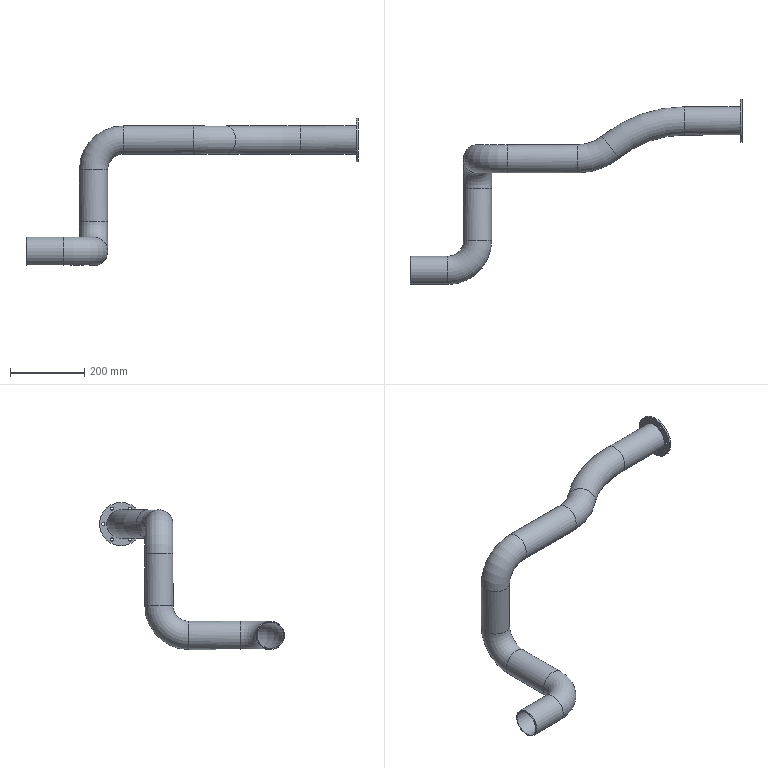Part | STEP file | Pipe Secondary Air | 1 solid | 31 faces | box 894.178 x 498.319 x 396.2 mm | volume 1004360 mm3 | cylinder 17 | torus 10 | plane 3 | cone 1 | commonest cylinder face diameters 8.376 x6 70.2 x5 76.2 x5 116.2 x1
STEP:
#1=CARTESIAN_POINT('',(-39.141,-4.548,-11.811));
#2=VERTEX_POINT('',#1);
#3=CARTESIAN_POINT('',(-39.141,-5.989,-11.811));
#4=DIRECTION('',(1.,0.,0.));
#5=DIRECTION('',(0.,-1.,0.));
#6=AXIS2_PLACEMENT_3D('',#3,#4,#5);
#7=CIRCLE('',#6,1.441);
#8=EDGE_CURVE('',#2,#2,#7,.T.);
#9=ORIENTED_EDGE('',*,*,#8,.T.);
#10=CARTESIAN_POINT('',(-39.082,-4.489,-11.811));
#11=VERTEX_POINT('',#10);
#12=CARTESIAN_POINT('',(-39.111,-4.518,-11.811));
#13=DIRECTION('',(0.7071,0.7071,0.));
#14=VECTOR('',#13,1.47);
#15=LINE('',#12,#14);
#16=EDGE_CURVE('',#2,#11,#15,.T.);
#17=ORIENTED_EDGE('',*,*,#16,.T.);
#18=CARTESIAN_POINT('',(-39.082,-7.489,-11.811));
#19=VERTEX_POINT('',#18);
#20=CARTESIAN_POINT('',(-39.082,-5.989,-11.811));
#21=DIRECTION('',(-1.,0.,0.));
#22=DIRECTION('',(0.,-1.,0.));
#23=AXIS2_PLACEMENT_3D('',#20,#21,#22);
#24=CIRCLE('',#23,1.5);
#25=EDGE_CURVE('',#11,#19,#24,.T.);
#26=ORIENTED_EDGE('',*,*,#25,.T.);
#27=CARTESIAN_POINT('',(-39.082,-5.989,-11.811));
#28=DIRECTION('',(-1.,0.,0.));
#29=DIRECTION('',(0.,-1.,0.));
#30=AXIS2_PLACEMENT_3D('',#27,#28,#29);
#31=CIRCLE('',#30,1.5);
#32=EDGE_CURVE('',#19,#11,#31,.T.);
#33=ORIENTED_EDGE('',*,*,#32,.T.);
#34=ORIENTED_EDGE('',*,*,#16,.F.);
#35=EDGE_LOOP('',(#9,#17,#26,#33,#34));
#36=FACE_OUTER_BOUND('',#35,.T.);
#37=CARTESIAN_POINT('',(-39.111,-5.989,-11.811));
#38=DIRECTION('',(1.,0.,0.));
#39=DIRECTION('',(0.,-1.,0.));
#40=AXIS2_PLACEMENT_3D('',#37,#38,#39);
#41=CONICAL_SURFACE('',#40,1.47,0.7854);
#42=ADVANCED_FACE('',(#36),#41,.T.);
#43=ORIENTED_EDGE('',*,*,#25,.F.);
#44=ORIENTED_EDGE('',*,*,#32,.F.);
#45=CARTESIAN_POINT('',(-35.125,-7.489,-11.811));
#46=VERTEX_POINT('',#45);
#47=CARTESIAN_POINT('',(-35.125,-7.489,-11.811));
#48=DIRECTION('',(1.,0.,0.));
#49=VECTOR('',#48,1.5);
#50=LINE('',#47,#49);
#51=EDGE_CURVE('',#19,#46,#50,.T.);
#52=ORIENTED_EDGE('',*,*,#51,.T.);
#53=CARTESIAN_POINT('',(-35.125,-4.489,-11.811));
#54=VERTEX_POINT('',#53);
#55=CARTESIAN_POINT('',(-35.125,-5.989,-11.811));
#56=DIRECTION('',(-1.,0.,0.));
#57=DIRECTION('',(0.,1.,0.));
#58=AXIS2_PLACEMENT_3D('',#55,#56,#57);
#59=CIRCLE('',#58,1.5);
#60=EDGE_CURVE('',#46,#54,#59,.T.);
#61=ORIENTED_EDGE('',*,*,#60,.T.);
#62=CARTESIAN_POINT('',(-35.125,-5.989,-11.811));
#63=DIRECTION('',(-1.,0.,0.));
#64=DIRECTION('',(0.,1.,0.));
#65=AXIS2_PLACEMENT_3D('',#62,#63,#64);
#66=CIRCLE('',#65,1.5);
#67=EDGE_CURVE('',#54,#46,#66,.T.);
#68=ORIENTED_EDGE('',*,*,#67,.T.);
#69=ORIENTED_EDGE('',*,*,#51,.F.);
#70=EDGE_LOOP('',(#43,#44,#52,#61,#68,#69));
#71=FACE_OUTER_BOUND('',#70,.T.);
#72=CARTESIAN_POINT('',(-35.125,-5.989,-11.811));
#73=DIRECTION('',(-1.,0.,0.));
#74=DIRECTION('',(0.,1.,0.));
#75=AXIS2_PLACEMENT_3D('',#72,#73,#74);
#76=CYLINDRICAL_SURFACE('',#75,1.5);
#77=ADVANCED_FACE('',(#71),#76,.T.);
#78=ORIENTED_EDGE('',*,*,#8,.F.);
#79=EDGE_LOOP('',(#78));
#80=FACE_OUTER_BOUND('',#79,.T.);
#81=CARTESIAN_POINT('',(-39.141,-4.607,-11.811));
#82=VERTEX_POINT('',#81);
#83=CARTESIAN_POINT('',(-39.141,-5.989,-11.811));
#84=DIRECTION('',(1.,0.,0.));
#85=DIRECTION('',(0.,-1.,0.));
#86=AXIS2_PLACEMENT_3D('',#83,#84,#85);
#87=CIRCLE('',#86,1.382);
#88=EDGE_CURVE('',#82,#82,#87,.T.);
#89=ORIENTED_EDGE('',*,*,#88,.T.);
#90=EDGE_LOOP('',(#89));
#91=FACE_BOUND('',#90,.T.);
#92=CARTESIAN_POINT('',(-39.141,-5.989,-11.811));
#93=DIRECTION('',(-1.,0.,0.));
#94=DIRECTION('',(0.,1.,0.));
#95=AXIS2_PLACEMENT_3D('',#92,#93,#94);
#96=PLANE('',#95);
#97=ADVANCED_FACE('',(#80,#91),#96,.T.);
#98=CARTESIAN_POINT('',(-35.125,-4.607,-11.811));
#99=VERTEX_POINT('',#98);
#100=CARTESIAN_POINT('',(-35.125,-5.989,-11.811));
#101=DIRECTION('',(-1.,0.,0.));
#102=DIRECTION('',(0.,-1.,0.));
#103=AXIS2_PLACEMENT_3D('',#100,#101,#102);
#104=CIRCLE('',#103,1.382);
#105=EDGE_CURVE('',#99,#99,#104,.T.);
#106=ORIENTED_EDGE('',*,*,#105,.F.);
#107=CARTESIAN_POINT('',(-35.125,-4.607,-11.811));
#108=DIRECTION('',(-1.,0.,0.));
#109=VECTOR('',#108,1.382);
#110=LINE('',#107,#109);
#111=EDGE_CURVE('',#99,#82,#110,.T.);
#112=ORIENTED_EDGE('',*,*,#111,.T.);
#113=ORIENTED_EDGE('',*,*,#88,.F.);
#114=ORIENTED_EDGE('',*,*,#111,.F.);
#115=EDGE_LOOP('',(#106,#112,#113,#114));
#116=FACE_OUTER_BOUND('',#115,.T.);
#117=CARTESIAN_POINT('',(-35.125,-5.989,-11.811));
#118=DIRECTION('',(-1.,0.,0.));
#119=DIRECTION('',(0.,-1.,0.));
#120=AXIS2_PLACEMENT_3D('',#117,#118,#119);
#121=CYLINDRICAL_SURFACE('',#120,1.382);
#122=ADVANCED_FACE('',(#116),#121,.F.);
#123=CARTESIAN_POINT('',(-33.357,-2.839,-11.811));
#124=VERTEX_POINT('',#123);
#125=CARTESIAN_POINT('',(-31.976,-2.839,-11.811));
#126=DIRECTION('',(0.,-1.,0.));
#127=DIRECTION('',(1.,0.,0.));
#128=AXIS2_PLACEMENT_3D('',#125,#126,#127);
#129=CIRCLE('',#128,1.382);
#130=EDGE_CURVE('',#124,#124,#129,.T.);
#131=ORIENTED_EDGE('',*,*,#130,.F.);
#132=CARTESIAN_POINT('',(-35.125,-2.839,-11.811));
#133=DIRECTION('',(0.,0.,-1.));
#134=DIRECTION('',(-1.,0.,0.));
#135=AXIS2_PLACEMENT_3D('',#132,#133,#134);
#136=CIRCLE('',#135,1.768);
#137=EDGE_CURVE('',#124,#99,#136,.T.);
#138=ORIENTED_EDGE('',*,*,#137,.T.);
#139=ORIENTED_EDGE('',*,*,#105,.T.);
#140=ORIENTED_EDGE('',*,*,#137,.F.);
#141=EDGE_LOOP('',(#131,#138,#139,#140));
#142=FACE_OUTER_BOUND('',#141,.T.);
#143=CARTESIAN_POINT('',(-35.125,-2.839,-11.811));
#144=DIRECTION('',(0.,0.,-1.));
#145=DIRECTION('',(-1.,0.,0.));
#146=AXIS2_PLACEMENT_3D('',#143,#144,#145);
#147=TOROIDAL_SURFACE('',#146,3.15,1.382);
#148=ADVANCED_FACE('',(#142),#147,.F.);
#149=CARTESIAN_POINT('',(-33.357,2.672,-11.811));
#150=VERTEX_POINT('',#149);
#151=CARTESIAN_POINT('',(-31.976,2.672,-10.429));
#152=VERTEX_POINT('',#151);
#153=CARTESIAN_POINT('',(-31.976,2.672,-11.811));
#154=DIRECTION('',(0.,-1.,0.));
#155=DIRECTION('',(1.,0.,0.));
#156=AXIS2_PLACEMENT_3D('',#153,#154,#155);
#157=CIRCLE('',#156,1.382);
#158=EDGE_CURVE('',#150,#152,#157,.T.);
#159=ORIENTED_EDGE('',*,*,#158,.F.);
#160=CARTESIAN_POINT('',(-33.357,2.672,-11.811));
#161=DIRECTION('',(0.,-1.,0.));
#162=VECTOR('',#161,1.382);
#163=LINE('',#160,#162);
#164=EDGE_CURVE('',#150,#124,#163,.T.);
#165=ORIENTED_EDGE('',*,*,#164,.T.);
#166=ORIENTED_EDGE('',*,*,#130,.T.);
#167=ORIENTED_EDGE('',*,*,#164,.F.);
#168=CARTESIAN_POINT('',(-31.976,2.672,-11.811));
#169=DIRECTION('',(0.,-1.,0.));
#170=DIRECTION('',(1.,0.,0.));
#171=AXIS2_PLACEMENT_3D('',#168,#169,#170);
#172=CIRCLE('',#171,1.382);
#173=EDGE_CURVE('',#152,#150,#172,.T.);
#174=ORIENTED_EDGE('',*,*,#173,.F.);
#175=EDGE_LOOP('',(#159,#165,#166,#167,#174));
#176=FACE_OUTER_BOUND('',#175,.T.);
#177=CARTESIAN_POINT('',(-31.976,2.672,-11.811));
#178=DIRECTION('',(0.,-1.,0.));
#179=DIRECTION('',(1.,0.,0.));
#180=AXIS2_PLACEMENT_3D('',#177,#178,#179);
#181=CYLINDRICAL_SURFACE('',#180,1.382);
#182=ADVANCED_FACE('',(#176),#181,.F.);
#183=CARTESIAN_POINT('',(-33.357,5.822,-8.661));
#184=VERTEX_POINT('',#183);
#185=CARTESIAN_POINT('',(-31.976,4.44,-8.661));
#186=VERTEX_POINT('',#185);
#187=CARTESIAN_POINT('',(-31.976,5.822,-8.661));
#188=DIRECTION('',(0.,0.,-1.));
#189=DIRECTION('',(1.,0.,0.));
#190=AXIS2_PLACEMENT_3D('',#187,#188,#189);
#191=CIRCLE('',#190,1.382);
#192=EDGE_CURVE('',#184,#186,#191,.T.);
#193=ORIENTED_EDGE('',*,*,#192,.F.);
#194=CARTESIAN_POINT('',(-31.976,5.822,-8.661));
#195=DIRECTION('',(0.,0.,-1.));
#196=DIRECTION('',(1.,0.,0.));
#197=AXIS2_PLACEMENT_3D('',#194,#195,#196);
#198=CIRCLE('',#197,1.382);
#199=EDGE_CURVE('',#186,#184,#198,.T.);
#200=ORIENTED_EDGE('',*,*,#199,.F.);
#201=CARTESIAN_POINT('',(-31.976,2.672,-8.661));
#202=DIRECTION('',(-1.,0.,0.));
#203=DIRECTION('',(0.,0.,1.));
#204=AXIS2_PLACEMENT_3D('',#201,#202,#203);
#205=CIRCLE('',#204,1.768);
#206=EDGE_CURVE('',#186,#152,#205,.T.);
#207=ORIENTED_EDGE('',*,*,#206,.T.);
#208=ORIENTED_EDGE('',*,*,#173,.T.);
#209=ORIENTED_EDGE('',*,*,#158,.T.);
#210=ORIENTED_EDGE('',*,*,#206,.F.);
#211=EDGE_LOOP('',(#193,#200,#207,#208,#209,#210));
#212=FACE_OUTER_BOUND('',#211,.T.);
#213=CARTESIAN_POINT('',(-31.976,2.672,-8.661));
#214=DIRECTION('',(-1.,0.,0.));
#215=DIRECTION('',(0.,0.,1.));
#216=AXIS2_PLACEMENT_3D('',#213,#214,#215);
#217=TOROIDAL_SURFACE('',#216,3.15,1.382);
#218=ADVANCED_FACE('',(#212),#217,.F.);
#219=CARTESIAN_POINT('',(-33.357,5.822,-3.15));
#220=VERTEX_POINT('',#219);
#221=CARTESIAN_POINT('',(-30.594,5.822,-3.15));
#222=VERTEX_POINT('',#221);
#223=CARTESIAN_POINT('',(-31.976,5.822,-3.15));
#224=DIRECTION('',(0.,0.,-1.));
#225=DIRECTION('',(1.,0.,0.));
#226=AXIS2_PLACEMENT_3D('',#223,#224,#225);
#227=CIRCLE('',#226,1.382);
#228=EDGE_CURVE('',#220,#222,#227,.T.);
#229=ORIENTED_EDGE('',*,*,#228,.F.);
#230=CARTESIAN_POINT('',(-33.357,5.822,-3.15));
#231=DIRECTION('',(0.,0.,-1.));
#232=VECTOR('',#231,1.382);
#233=LINE('',#230,#232);
#234=EDGE_CURVE('',#220,#184,#233,.T.);
#235=ORIENTED_EDGE('',*,*,#234,.T.);
#236=ORIENTED_EDGE('',*,*,#192,.T.);
#237=ORIENTED_EDGE('',*,*,#199,.T.);
#238=ORIENTED_EDGE('',*,*,#234,.F.);
#239=CARTESIAN_POINT('',(-31.976,5.822,-3.15));
#240=DIRECTION('',(0.,0.,-1.));
#241=DIRECTION('',(1.,0.,0.));
#242=AXIS2_PLACEMENT_3D('',#239,#240,#241);
#243=CIRCLE('',#242,1.382);
#244=EDGE_CURVE('',#222,#220,#243,.T.);
#245=ORIENTED_EDGE('',*,*,#244,.F.);
#246=EDGE_LOOP('',(#229,#235,#236,#237,#238,#245));
#247=FACE_OUTER_BOUND('',#246,.T.);
#248=CARTESIAN_POINT('',(-31.976,5.822,-3.15));
#249=DIRECTION('',(0.,0.,-1.));
#250=DIRECTION('',(1.,0.,0.));
#251=AXIS2_PLACEMENT_3D('',#248,#249,#250);
#252=CYLINDRICAL_SURFACE('',#251,1.382);
#253=ADVANCED_FACE('',(#247),#252,.F.);
#254=CARTESIAN_POINT('',(-28.826,5.822,1.382));
#255=VERTEX_POINT('',#254);
#256=CARTESIAN_POINT('',(-28.826,5.822,-1.382));
#257=VERTEX_POINT('',#256);
#258=CARTESIAN_POINT('',(-28.826,5.822,0.));
#259=DIRECTION('',(-1.,0.,0.));
#260=DIRECTION('',(0.,0.,-1.));
#261=AXIS2_PLACEMENT_3D('',#258,#259,#260);
#262=CIRCLE('',#261,1.382);
#263=EDGE_CURVE('',#255,#257,#262,.T.);
#264=ORIENTED_EDGE('',*,*,#263,.F.);
#265=CARTESIAN_POINT('',(-28.826,5.822,0.));
#266=DIRECTION('',(-1.,0.,0.));
#267=DIRECTION('',(0.,0.,-1.));
#268=AXIS2_PLACEMENT_3D('',#265,#266,#267);
#269=CIRCLE('',#268,1.382);
#270=EDGE_CURVE('',#257,#255,#269,.T.);
#271=ORIENTED_EDGE('',*,*,#270,.F.);
#272=CARTESIAN_POINT('',(-28.826,5.822,-3.15));
#273=DIRECTION('',(0.,-1.,0.));
#274=DIRECTION('',(0.,0.,-1.));
#275=AXIS2_PLACEMENT_3D('',#272,#273,#274);
#276=CIRCLE('',#275,1.768);
#277=EDGE_CURVE('',#257,#222,#276,.T.);
#278=ORIENTED_EDGE('',*,*,#277,.T.);
#279=ORIENTED_EDGE('',*,*,#244,.T.);
#280=ORIENTED_EDGE('',*,*,#228,.T.);
#281=ORIENTED_EDGE('',*,*,#277,.F.);
#282=EDGE_LOOP('',(#264,#271,#278,#279,#280,#281));
#283=FACE_OUTER_BOUND('',#282,.T.);
#284=CARTESIAN_POINT('',(-28.826,5.822,-3.15));
#285=DIRECTION('',(0.,-1.,0.));
#286=DIRECTION('',(0.,0.,-1.));
#287=AXIS2_PLACEMENT_3D('',#284,#285,#286);
#288=TOROIDAL_SURFACE('',#287,3.15,1.382);
#289=ADVANCED_FACE('',(#283),#288,.F.);
#290=ORIENTED_EDGE('',*,*,#67,.F.);
#291=CARTESIAN_POINT('',(-33.476,-2.839,-11.811));
#292=VERTEX_POINT('',#291);
#293=CARTESIAN_POINT('',(-35.125,-2.839,-11.811));
#294=DIRECTION('',(0.,0.,1.));
#295=DIRECTION('',(-1.,0.,0.));
#296=AXIS2_PLACEMENT_3D('',#293,#294,#295);
#297=CIRCLE('',#296,1.65);
#298=EDGE_CURVE('',#54,#292,#297,.T.);
#299=ORIENTED_EDGE('',*,*,#298,.T.);
#300=CARTESIAN_POINT('',(-30.476,-2.839,-11.811));
#301=VERTEX_POINT('',#300);
#302=CARTESIAN_POINT('',(-31.976,-2.839,-11.811));
#303=DIRECTION('',(0.,-1.,0.));
#304=DIRECTION('',(-1.,0.,0.));
#305=AXIS2_PLACEMENT_3D('',#302,#303,#304);
#306=CIRCLE('',#305,1.5);
#307=EDGE_CURVE('',#292,#301,#306,.T.);
#308=ORIENTED_EDGE('',*,*,#307,.T.);
#309=CARTESIAN_POINT('',(-31.976,-2.839,-11.811));
#310=DIRECTION('',(0.,-1.,0.));
#311=DIRECTION('',(-1.,0.,0.));
#312=AXIS2_PLACEMENT_3D('',#309,#310,#311);
#313=CIRCLE('',#312,1.5);
#314=EDGE_CURVE('',#301,#292,#313,.T.);
#315=ORIENTED_EDGE('',*,*,#314,.T.);
#316=ORIENTED_EDGE('',*,*,#298,.F.);
#317=ORIENTED_EDGE('',*,*,#60,.F.);
#318=EDGE_LOOP('',(#290,#299,#308,#315,#316,#317));
#319=FACE_OUTER_BOUND('',#318,.T.);
#320=CARTESIAN_POINT('',(-35.125,-2.839,-11.811));
#321=DIRECTION('',(0.,0.,-1.));
#322=DIRECTION('',(-1.,0.,0.));
#323=AXIS2_PLACEMENT_3D('',#320,#321,#322);
#324=TOROIDAL_SURFACE('',#323,3.15,1.5);
#325=ADVANCED_FACE('',(#319),#324,.T.);
#326=ORIENTED_EDGE('',*,*,#307,.F.);
#327=ORIENTED_EDGE('',*,*,#314,.F.);
#328=CARTESIAN_POINT('',(-30.476,2.672,-11.811));
#329=VERTEX_POINT('',#328);
#330=CARTESIAN_POINT('',(-30.476,2.672,-11.811));
#331=DIRECTION('',(0.,1.,0.));
#332=VECTOR('',#331,1.5);
#333=LINE('',#330,#332);
#334=EDGE_CURVE('',#301,#329,#333,.T.);
#335=ORIENTED_EDGE('',*,*,#334,.T.);
#336=CARTESIAN_POINT('',(-31.976,2.672,-10.311));
#337=VERTEX_POINT('',#336);
#338=CARTESIAN_POINT('',(-31.976,2.672,-11.811));
#339=DIRECTION('',(0.,-1.,0.));
#340=DIRECTION('',(-1.,0.,0.));
#341=AXIS2_PLACEMENT_3D('',#338,#339,#340);
#342=CIRCLE('',#341,1.5);
#343=EDGE_CURVE('',#329,#337,#342,.T.);
#344=ORIENTED_EDGE('',*,*,#343,.T.);
#345=CARTESIAN_POINT('',(-31.976,2.672,-11.811));
#346=DIRECTION('',(0.,-1.,0.));
#347=DIRECTION('',(-1.,0.,0.));
#348=AXIS2_PLACEMENT_3D('',#345,#346,#347);
#349=CIRCLE('',#348,1.5);
#350=EDGE_CURVE('',#337,#329,#349,.T.);
#351=ORIENTED_EDGE('',*,*,#350,.T.);
#352=ORIENTED_EDGE('',*,*,#334,.F.);
#353=EDGE_LOOP('',(#326,#327,#335,#344,#351,#352));
#354=FACE_OUTER_BOUND('',#353,.T.);
#355=CARTESIAN_POINT('',(-31.976,2.672,-11.811));
#356=DIRECTION('',(0.,-1.,0.));
#357=DIRECTION('',(-1.,0.,0.));
#358=AXIS2_PLACEMENT_3D('',#355,#356,#357);
#359=CYLINDRICAL_SURFACE('',#358,1.5);
#360=ADVANCED_FACE('',(#354),#359,.T.);
#361=ORIENTED_EDGE('',*,*,#350,.F.);
#362=CARTESIAN_POINT('',(-31.976,4.322,-8.661));
#363=VERTEX_POINT('',#362);
#364=CARTESIAN_POINT('',(-31.976,2.672,-8.661));
#365=DIRECTION('',(1.,0.,0.));
#366=DIRECTION('',(0.,0.,1.));
#367=AXIS2_PLACEMENT_3D('',#364,#365,#366);
#368=CIRCLE('',#367,1.65);
#369=EDGE_CURVE('',#337,#363,#368,.T.);
#370=ORIENTED_EDGE('',*,*,#369,.T.);
#371=CARTESIAN_POINT('',(-30.476,5.822,-8.661));
#372=VERTEX_POINT('',#371);
#373=CARTESIAN_POINT('',(-31.976,5.822,-8.661));
#374=DIRECTION('',(0.,0.,-1.));
#375=DIRECTION('',(-1.,0.,0.));
#376=AXIS2_PLACEMENT_3D('',#373,#374,#375);
#377=CIRCLE('',#376,1.5);
#378=EDGE_CURVE('',#363,#372,#377,.T.);
#379=ORIENTED_EDGE('',*,*,#378,.T.);
#380=CARTESIAN_POINT('',(-31.976,5.822,-8.661));
#381=DIRECTION('',(0.,0.,-1.));
#382=DIRECTION('',(-1.,0.,0.));
#383=AXIS2_PLACEMENT_3D('',#380,#381,#382);
#384=CIRCLE('',#383,1.5);
#385=EDGE_CURVE('',#372,#363,#384,.T.);
#386=ORIENTED_EDGE('',*,*,#385,.T.);
#387=ORIENTED_EDGE('',*,*,#369,.F.);
#388=ORIENTED_EDGE('',*,*,#343,.F.);
#389=EDGE_LOOP('',(#361,#370,#379,#386,#387,#388));
#390=FACE_OUTER_BOUND('',#389,.T.);
#391=CARTESIAN_POINT('',(-31.976,2.672,-8.661));
#392=DIRECTION('',(-1.,0.,0.));
#393=DIRECTION('',(0.,0.,1.));
#394=AXIS2_PLACEMENT_3D('',#391,#392,#393);
#395=TOROIDAL_SURFACE('',#394,3.15,1.5);
#396=ADVANCED_FACE('',(#390),#395,.T.);
#397=ORIENTED_EDGE('',*,*,#378,.F.);
#398=ORIENTED_EDGE('',*,*,#385,.F.);
#399=CARTESIAN_POINT('',(-30.476,5.822,-3.15));
#400=VERTEX_POINT('',#399);
#401=CARTESIAN_POINT('',(-30.476,5.822,-3.15));
#402=DIRECTION('',(0.,0.,1.));
#403=VECTOR('',#402,1.5);
#404=LINE('',#401,#403);
#405=EDGE_CURVE('',#372,#400,#404,.T.);
#406=ORIENTED_EDGE('',*,*,#405,.T.);
#407=CARTESIAN_POINT('',(-31.976,5.822,-3.15));
#408=DIRECTION('',(0.,0.,-1.));
#409=DIRECTION('',(-1.,0.,0.));
#410=AXIS2_PLACEMENT_3D('',#407,#408,#409);
#411=CIRCLE('',#410,1.5);
#412=EDGE_CURVE('',#400,#400,#411,.T.);
#413=ORIENTED_EDGE('',*,*,#412,.T.);
#414=ORIENTED_EDGE('',*,*,#405,.F.);
#415=EDGE_LOOP('',(#397,#398,#406,#413,#414));
#416=FACE_OUTER_BOUND('',#415,.T.);
#417=CARTESIAN_POINT('',(-31.976,5.822,-3.15));
#418=DIRECTION('',(0.,0.,-1.));
#419=DIRECTION('',(-1.,0.,0.));
#420=AXIS2_PLACEMENT_3D('',#417,#418,#419);
#421=CYLINDRICAL_SURFACE('',#420,1.5);
#422=ADVANCED_FACE('',(#416),#421,.T.);
#423=ORIENTED_EDGE('',*,*,#412,.F.);
#424=CARTESIAN_POINT('',(-28.826,5.822,-1.5));
#425=VERTEX_POINT('',#424);
#426=CARTESIAN_POINT('',(-28.826,5.822,-3.15));
#427=DIRECTION('',(0.,1.,0.));
#428=DIRECTION('',(0.,0.,-1.));
#429=AXIS2_PLACEMENT_3D('',#426,#427,#428);
#430=CIRCLE('',#429,1.65);
#431=EDGE_CURVE('',#400,#425,#430,.T.);
#432=ORIENTED_EDGE('',*,*,#431,.T.);
#433=CARTESIAN_POINT('',(-28.826,5.822,0.));
#434=DIRECTION('',(-1.,0.,0.));
#435=DIRECTION('',(0.,0.,1.));
#436=AXIS2_PLACEMENT_3D('',#433,#434,#435);
#437=CIRCLE('',#436,1.5);
#438=EDGE_CURVE('',#425,#425,#437,.T.);
#439=ORIENTED_EDGE('',*,*,#438,.T.);
#440=ORIENTED_EDGE('',*,*,#431,.F.);
#441=EDGE_LOOP('',(#423,#432,#439,#440));
#442=FACE_OUTER_BOUND('',#441,.T.);
#443=CARTESIAN_POINT('',(-28.826,5.822,-3.15));
#444=DIRECTION('',(0.,-1.,0.));
#445=DIRECTION('',(0.,0.,-1.));
#446=AXIS2_PLACEMENT_3D('',#443,#444,#445);
#447=TOROIDAL_SURFACE('',#446,3.15,1.5);
#448=ADVANCED_FACE('',(#442),#447,.T.);
#449=CARTESIAN_POINT('',(-21.348,5.822,1.382));
#450=VERTEX_POINT('',#449);
#451=CARTESIAN_POINT('',(-21.348,7.204,0.));
#452=VERTEX_POINT('',#451);
#453=CARTESIAN_POINT('',(-21.348,5.822,0.));
#454=DIRECTION('',(-1.,0.,0.));
#455=DIRECTION('',(0.,0.,-1.));
#456=AXIS2_PLACEMENT_3D('',#453,#454,#455);
#457=CIRCLE('',#456,1.382);
#458=EDGE_CURVE('',#450,#452,#457,.T.);
#459=ORIENTED_EDGE('',*,*,#458,.F.);
#460=CARTESIAN_POINT('',(-21.348,5.822,1.382));
#461=DIRECTION('',(-1.,0.,0.));
#462=VECTOR('',#461,1.382);
#463=LINE('',#460,#462);
#464=EDGE_CURVE('',#450,#255,#463,.T.);
#465=ORIENTED_EDGE('',*,*,#464,.T.);
#466=ORIENTED_EDGE('',*,*,#263,.T.);
#467=ORIENTED_EDGE('',*,*,#270,.T.);
#468=ORIENTED_EDGE('',*,*,#464,.F.);
#469=CARTESIAN_POINT('',(-21.348,5.822,0.));
#470=DIRECTION('',(-1.,0.,0.));
#471=DIRECTION('',(0.,0.,-1.));
#472=AXIS2_PLACEMENT_3D('',#469,#470,#471);
#473=CIRCLE('',#472,1.382);
#474=EDGE_CURVE('',#452,#450,#473,.T.);
#475=ORIENTED_EDGE('',*,*,#474,.F.);
#476=EDGE_LOOP('',(#459,#465,#466,#467,#468,#475));
#477=FACE_OUTER_BOUND('',#476,.T.);
#478=CARTESIAN_POINT('',(-21.348,5.822,0.));
#479=DIRECTION('',(-1.,0.,0.));
#480=DIRECTION('',(0.,0.,-1.));
#481=AXIS2_PLACEMENT_3D('',#478,#479,#480);
#482=CYLINDRICAL_SURFACE('',#481,1.382);
#483=ADVANCED_FACE('',(#477),#482,.F.);
#484=CARTESIAN_POINT('',(-16.996,5.987,0.));
#485=VERTEX_POINT('',#484);
#486=CARTESIAN_POINT('',(-18.74,8.131,0.));
#487=VERTEX_POINT('',#486);
#488=CARTESIAN_POINT('',(-17.868,7.059,0.));
#489=DIRECTION('',(-0.7756,-0.6313,0.));
#490=DIRECTION('',(0.,0.,-1.));
#491=AXIS2_PLACEMENT_3D('',#488,#489,#490);
#492=CIRCLE('',#491,1.382);
#493=EDGE_CURVE('',#485,#487,#492,.T.);
#494=ORIENTED_EDGE('',*,*,#493,.F.);
#495=CARTESIAN_POINT('',(-17.868,7.059,0.));
#496=DIRECTION('',(-0.7756,-0.6313,0.));
#497=DIRECTION('',(0.,0.,-1.));
#498=AXIS2_PLACEMENT_3D('',#495,#496,#497);
#499=CIRCLE('',#498,1.382);
#500=EDGE_CURVE('',#487,#485,#499,.T.);
#501=ORIENTED_EDGE('',*,*,#500,.F.);
#502=CARTESIAN_POINT('',(-21.348,11.334,0.));
#503=DIRECTION('',(0.,0.,-1.));
#504=DIRECTION('',(-1.,0.,0.));
#505=AXIS2_PLACEMENT_3D('',#502,#503,#504);
#506=CIRCLE('',#505,4.13);
#507=EDGE_CURVE('',#487,#452,#506,.T.);
#508=ORIENTED_EDGE('',*,*,#507,.T.);
#509=ORIENTED_EDGE('',*,*,#474,.T.);
#510=ORIENTED_EDGE('',*,*,#458,.T.);
#511=ORIENTED_EDGE('',*,*,#507,.F.);
#512=EDGE_LOOP('',(#494,#501,#508,#509,#510,#511));
#513=FACE_OUTER_BOUND('',#512,.T.);
#514=CARTESIAN_POINT('',(-21.348,11.334,0.));
#515=DIRECTION('',(0.,0.,-1.));
#516=DIRECTION('',(-1.,0.,0.));
#517=AXIS2_PLACEMENT_3D('',#514,#515,#516);
#518=TOROIDAL_SURFACE('',#517,5.512,1.382);
#519=ADVANCED_FACE('',(#513),#518,.F.);
#520=CARTESIAN_POINT('',(-10.039,9.843,1.382));
#521=VERTEX_POINT('',#520);
#522=CARTESIAN_POINT('',(-10.039,8.461,0.));
#523=VERTEX_POINT('',#522);
#524=CARTESIAN_POINT('',(-10.039,9.843,0.));
#525=DIRECTION('',(-1.,0.,0.));
#526=DIRECTION('',(0.,0.,-1.));
#527=AXIS2_PLACEMENT_3D('',#524,#525,#526);
#528=CIRCLE('',#527,1.382);
#529=EDGE_CURVE('',#521,#523,#528,.T.);
#530=ORIENTED_EDGE('',*,*,#529,.F.);
#531=CARTESIAN_POINT('',(-10.039,9.843,0.));
#532=DIRECTION('',(-1.,0.,0.));
#533=DIRECTION('',(0.,0.,-1.));
#534=AXIS2_PLACEMENT_3D('',#531,#532,#533);
#535=CIRCLE('',#534,1.382);
#536=EDGE_CURVE('',#523,#521,#535,.T.);
#537=ORIENTED_EDGE('',*,*,#536,.F.);
#538=CARTESIAN_POINT('',(-10.039,-2.559,0.));
#539=DIRECTION('',(0.,0.,1.));
#540=DIRECTION('',(1.,0.,0.));
#541=AXIS2_PLACEMENT_3D('',#538,#539,#540);
#542=CIRCLE('',#541,11.02);
#543=EDGE_CURVE('',#523,#485,#542,.T.);
#544=ORIENTED_EDGE('',*,*,#543,.T.);
#545=ORIENTED_EDGE('',*,*,#493,.T.);
#546=ORIENTED_EDGE('',*,*,#500,.T.);
#547=ORIENTED_EDGE('',*,*,#543,.F.);
#548=EDGE_LOOP('',(#530,#537,#544,#545,#546,#547));
#549=FACE_OUTER_BOUND('',#548,.T.);
#550=CARTESIAN_POINT('',(-10.039,-2.559,0.));
#551=DIRECTION('',(0.,0.,1.));
#552=DIRECTION('',(1.,0.,0.));
#553=AXIS2_PLACEMENT_3D('',#550,#551,#552);
#554=TOROIDAL_SURFACE('',#553,12.402,1.382);
#555=ADVANCED_FACE('',(#549),#554,.F.);
#556=ORIENTED_EDGE('',*,*,#438,.F.);
#557=CARTESIAN_POINT('',(-21.348,5.822,-1.5));
#558=VERTEX_POINT('',#557);
#559=CARTESIAN_POINT('',(-21.348,5.822,-1.5));
#560=DIRECTION('',(1.,0.,0.));
#561=VECTOR('',#560,1.5);
#562=LINE('',#559,#561);
#563=EDGE_CURVE('',#425,#558,#562,.T.);
#564=ORIENTED_EDGE('',*,*,#563,.T.);
#565=CARTESIAN_POINT('',(-21.348,7.322,0.));
#566=VERTEX_POINT('',#565);
#567=CARTESIAN_POINT('',(-21.348,5.822,0.));
#568=DIRECTION('',(-1.,0.,0.));
#569=DIRECTION('',(0.,0.,1.));
#570=AXIS2_PLACEMENT_3D('',#567,#568,#569);
#571=CIRCLE('',#570,1.5);
#572=EDGE_CURVE('',#558,#566,#571,.T.);
#573=ORIENTED_EDGE('',*,*,#572,.T.);
#574=CARTESIAN_POINT('',(-21.348,5.822,0.));
#575=DIRECTION('',(-1.,0.,0.));
#576=DIRECTION('',(0.,0.,1.));
#577=AXIS2_PLACEMENT_3D('',#574,#575,#576);
#578=CIRCLE('',#577,1.5);
#579=EDGE_CURVE('',#566,#558,#578,.T.);
#580=ORIENTED_EDGE('',*,*,#579,.T.);
#581=ORIENTED_EDGE('',*,*,#563,.F.);
#582=EDGE_LOOP('',(#556,#564,#573,#580,#581));
#583=FACE_OUTER_BOUND('',#582,.T.);
#584=CARTESIAN_POINT('',(-21.348,5.822,0.));
#585=DIRECTION('',(-1.,0.,0.));
#586=DIRECTION('',(0.,0.,1.));
#587=AXIS2_PLACEMENT_3D('',#584,#585,#586);
#588=CYLINDRICAL_SURFACE('',#587,1.5);
#589=ADVANCED_FACE('',(#583),#588,.T.);
#590=ORIENTED_EDGE('',*,*,#572,.F.);
#591=ORIENTED_EDGE('',*,*,#579,.F.);
#592=CARTESIAN_POINT('',(-18.815,8.222,0.));
#593=VERTEX_POINT('',#592);
#594=CARTESIAN_POINT('',(-21.348,11.334,0.));
#595=DIRECTION('',(0.,0.,1.));
#596=DIRECTION('',(-1.,0.,0.));
#597=AXIS2_PLACEMENT_3D('',#594,#595,#596);
#598=CIRCLE('',#597,4.012);
#599=EDGE_CURVE('',#566,#593,#598,.T.);
#600=ORIENTED_EDGE('',*,*,#599,.T.);
#601=CARTESIAN_POINT('',(-16.921,5.896,0.));
#602=VERTEX_POINT('',#601);
#603=CARTESIAN_POINT('',(-17.868,7.059,0.));
#604=DIRECTION('',(-0.7756,-0.6313,0.));
#605=DIRECTION('',(0.,0.,1.));
#606=AXIS2_PLACEMENT_3D('',#603,#604,#605);
#607=CIRCLE('',#606,1.5);
#608=EDGE_CURVE('',#593,#602,#607,.T.);
#609=ORIENTED_EDGE('',*,*,#608,.T.);
#610=CARTESIAN_POINT('',(-17.868,7.059,0.));
#611=DIRECTION('',(-0.7756,-0.6313,0.));
#612=DIRECTION('',(0.,0.,1.));
#613=AXIS2_PLACEMENT_3D('',#610,#611,#612);
#614=CIRCLE('',#613,1.5);
#615=EDGE_CURVE('',#602,#593,#614,.T.);
#616=ORIENTED_EDGE('',*,*,#615,.T.);
#617=ORIENTED_EDGE('',*,*,#599,.F.);
#618=EDGE_LOOP('',(#590,#591,#600,#609,#616,#617));
#619=FACE_OUTER_BOUND('',#618,.T.);
#620=CARTESIAN_POINT('',(-21.348,11.334,0.));
#621=DIRECTION('',(0.,0.,-1.));
#622=DIRECTION('',(-1.,0.,0.));
#623=AXIS2_PLACEMENT_3D('',#620,#621,#622);
#624=TOROIDAL_SURFACE('',#623,5.512,1.5);
#625=ADVANCED_FACE('',(#619),#624,.T.);
#626=ORIENTED_EDGE('',*,*,#615,.F.);
#627=CARTESIAN_POINT('',(-10.039,8.343,0.));
#628=VERTEX_POINT('',#627);
#629=CARTESIAN_POINT('',(-10.039,-2.559,0.));
#630=DIRECTION('',(0.,0.,-1.));
#631=DIRECTION('',(1.,0.,0.));
#632=AXIS2_PLACEMENT_3D('',#629,#630,#631);
#633=CIRCLE('',#632,10.902);
#634=EDGE_CURVE('',#602,#628,#633,.T.);
#635=ORIENTED_EDGE('',*,*,#634,.T.);
#636=CARTESIAN_POINT('',(-10.039,9.843,-1.5));
#637=VERTEX_POINT('',#636);
#638=CARTESIAN_POINT('',(-10.039,9.843,0.));
#639=DIRECTION('',(-1.,0.,0.));
#640=DIRECTION('',(0.,0.,1.));
#641=AXIS2_PLACEMENT_3D('',#638,#639,#640);
#642=CIRCLE('',#641,1.5);
#643=EDGE_CURVE('',#628,#637,#642,.T.);
#644=ORIENTED_EDGE('',*,*,#643,.T.);
#645=CARTESIAN_POINT('',(-10.039,9.843,0.));
#646=DIRECTION('',(-1.,0.,0.));
#647=DIRECTION('',(0.,0.,1.));
#648=AXIS2_PLACEMENT_3D('',#645,#646,#647);
#649=CIRCLE('',#648,1.5);
#650=EDGE_CURVE('',#637,#628,#649,.T.);
#651=ORIENTED_EDGE('',*,*,#650,.T.);
#652=ORIENTED_EDGE('',*,*,#634,.F.);
#653=ORIENTED_EDGE('',*,*,#608,.F.);
#654=EDGE_LOOP('',(#626,#635,#644,#651,#652,#653));
#655=FACE_OUTER_BOUND('',#654,.T.);
#656=CARTESIAN_POINT('',(-10.039,-2.559,0.));
#657=DIRECTION('',(0.,0.,1.));
#658=DIRECTION('',(1.,0.,0.));
#659=AXIS2_PLACEMENT_3D('',#656,#657,#658);
#660=TOROIDAL_SURFACE('',#659,12.402,1.5);
#661=ADVANCED_FACE('',(#655),#660,.T.);
#662=ORIENTED_EDGE('',*,*,#643,.F.);
#663=ORIENTED_EDGE('',*,*,#650,.F.);
#664=CARTESIAN_POINT('',(-4.134,9.843,-1.5));
#665=VERTEX_POINT('',#664);
#666=CARTESIAN_POINT('',(-4.134,9.843,-1.5));
#667=DIRECTION('',(1.,0.,0.));
#668=VECTOR('',#667,1.5);
#669=LINE('',#666,#668);
#670=EDGE_CURVE('',#637,#665,#669,.T.);
#671=ORIENTED_EDGE('',*,*,#670,.T.);
#672=CARTESIAN_POINT('',(-4.134,9.843,0.));
#673=DIRECTION('',(1.,0.,0.));
#674=DIRECTION('',(0.,0.,1.));
#675=AXIS2_PLACEMENT_3D('',#672,#673,#674);
#676=CIRCLE('',#675,1.5);
#677=EDGE_CURVE('',#665,#665,#676,.T.);
#678=ORIENTED_EDGE('',*,*,#677,.F.);
#679=ORIENTED_EDGE('',*,*,#670,.F.);
#680=EDGE_LOOP('',(#662,#663,#671,#678,#679));
#681=FACE_OUTER_BOUND('',#680,.T.);
#682=CARTESIAN_POINT('',(-4.134,9.843,0.));
#683=DIRECTION('',(-1.,0.,0.));
#684=DIRECTION('',(0.,0.,1.));
#685=AXIS2_PLACEMENT_3D('',#682,#683,#684);
#686=CYLINDRICAL_SURFACE('',#685,1.5);
#687=ADVANCED_FACE('',(#681),#686,.T.);
#688=CARTESIAN_POINT('',(-4.134,10.932,1.558));
#689=VERTEX_POINT('',#688);
#690=CARTESIAN_POINT('',(-4.134,10.789,1.64));
#691=DIRECTION('',(1.,0.,0.));
#692=DIRECTION('',(0.,-0.866,0.5));
#693=AXIS2_PLACEMENT_3D('',#690,#691,#692);
#694=CIRCLE('',#693,0.1649);
#695=EDGE_CURVE('',#689,#689,#694,.T.);
#696=ORIENTED_EDGE('',*,*,#695,.F.);
#697=CARTESIAN_POINT('',(-3.937,10.932,1.558));
#698=VERTEX_POINT('',#697);
#699=CARTESIAN_POINT('',(-4.035,10.932,1.558));
#700=DIRECTION('',(1.,0.,0.));
#701=VECTOR('',#700,0.1649);
#702=LINE('',#699,#701);
#703=EDGE_CURVE('',#689,#698,#702,.T.);
#704=ORIENTED_EDGE('',*,*,#703,.T.);
#705=CARTESIAN_POINT('',(-3.937,10.789,1.64));
#706=DIRECTION('',(-1.,0.,0.));
#707=DIRECTION('',(0.,-0.866,0.5));
#708=AXIS2_PLACEMENT_3D('',#705,#706,#707);
#709=CIRCLE('',#708,0.1649);
#710=EDGE_CURVE('',#698,#698,#709,.T.);
#711=ORIENTED_EDGE('',*,*,#710,.F.);
#712=ORIENTED_EDGE('',*,*,#703,.F.);
#713=EDGE_LOOP('',(#696,#704,#711,#712));
#714=FACE_OUTER_BOUND('',#713,.T.);
#715=CARTESIAN_POINT('',(-4.035,10.789,1.64));
#716=DIRECTION('',(-1.,0.,0.));
#717=DIRECTION('',(0.,-0.866,0.5));
#718=AXIS2_PLACEMENT_3D('',#715,#716,#717);
#719=CYLINDRICAL_SURFACE('',#718,0.1649);
#720=ADVANCED_FACE('',(#714),#719,.F.);
#721=CARTESIAN_POINT('',(-4.134,9.038,1.722));
#722=VERTEX_POINT('',#721);
#723=CARTESIAN_POINT('',(-4.134,8.896,1.64));
#724=DIRECTION('',(1.,0.,0.));
#725=DIRECTION('',(0.,-0.866,-0.5));
#726=AXIS2_PLACEMENT_3D('',#723,#724,#725);
#727=CIRCLE('',#726,0.1649);
#728=EDGE_CURVE('',#722,#722,#727,.T.);
#729=ORIENTED_EDGE('',*,*,#728,.F.);
#730=CARTESIAN_POINT('',(-3.937,9.038,1.722));
#731=VERTEX_POINT('',#730);
#732=CARTESIAN_POINT('',(-4.035,9.038,1.722));
#733=DIRECTION('',(1.,0.,0.));
#734=VECTOR('',#733,0.1649);
#735=LINE('',#732,#734);
#736=EDGE_CURVE('',#722,#731,#735,.T.);
#737=ORIENTED_EDGE('',*,*,#736,.T.);
#738=CARTESIAN_POINT('',(-3.937,8.896,1.64));
#739=DIRECTION('',(-1.,0.,0.));
#740=DIRECTION('',(0.,-0.866,-0.5));
#741=AXIS2_PLACEMENT_3D('',#738,#739,#740);
#742=CIRCLE('',#741,0.1649);
#743=EDGE_CURVE('',#731,#731,#742,.T.);
#744=ORIENTED_EDGE('',*,*,#743,.F.);
#745=ORIENTED_EDGE('',*,*,#736,.F.);
#746=EDGE_LOOP('',(#729,#737,#744,#745));
#747=FACE_OUTER_BOUND('',#746,.T.);
#748=CARTESIAN_POINT('',(-4.035,8.896,1.64));
#749=DIRECTION('',(-1.,0.,0.));
#750=DIRECTION('',(0.,-0.866,-0.5));
#751=AXIS2_PLACEMENT_3D('',#748,#749,#750);
#752=CYLINDRICAL_SURFACE('',#751,0.1649);
#753=ADVANCED_FACE('',(#747),#752,.F.);
#754=CARTESIAN_POINT('',(-4.134,7.949,0.1649));
#755=VERTEX_POINT('',#754);
#756=CARTESIAN_POINT('',(-4.134,7.949,0.));
#757=DIRECTION('',(1.,0.,0.));
#758=DIRECTION('',(0.,0.,-1.));
#759=AXIS2_PLACEMENT_3D('',#756,#757,#758);
#760=CIRCLE('',#759,0.1649);
#761=EDGE_CURVE('',#755,#755,#760,.T.);
#762=ORIENTED_EDGE('',*,*,#761,.F.);
#763=CARTESIAN_POINT('',(-3.937,7.949,0.1649));
#764=VERTEX_POINT('',#763);
#765=CARTESIAN_POINT('',(-4.035,7.949,0.1649));
#766=DIRECTION('',(1.,0.,0.));
#767=VECTOR('',#766,0.1649);
#768=LINE('',#765,#767);
#769=EDGE_CURVE('',#755,#764,#768,.T.);
#770=ORIENTED_EDGE('',*,*,#769,.T.);
#771=CARTESIAN_POINT('',(-3.937,7.949,0.));
#772=DIRECTION('',(-1.,0.,0.));
#773=DIRECTION('',(0.,0.,-1.));
#774=AXIS2_PLACEMENT_3D('',#771,#772,#773);
#775=CIRCLE('',#774,0.1649);
#776=EDGE_CURVE('',#764,#764,#775,.T.);
#777=ORIENTED_EDGE('',*,*,#776,.F.);
#778=ORIENTED_EDGE('',*,*,#769,.F.);
#779=EDGE_LOOP('',(#762,#770,#777,#778));
#780=FACE_OUTER_BOUND('',#779,.T.);
#781=CARTESIAN_POINT('',(-4.035,7.949,0.));
#782=DIRECTION('',(-1.,0.,0.));
#783=DIRECTION('',(0.,0.,-1.));
#784=AXIS2_PLACEMENT_3D('',#781,#782,#783);
#785=CYLINDRICAL_SURFACE('',#784,0.1649);
#786=ADVANCED_FACE('',(#780),#785,.F.);
#787=CARTESIAN_POINT('',(-4.134,8.753,-1.558));
#788=VERTEX_POINT('',#787);
#789=CARTESIAN_POINT('',(-4.134,8.896,-1.64));
#790=DIRECTION('',(1.,0.,0.));
#791=DIRECTION('',(0.,0.866,-0.5));
#792=AXIS2_PLACEMENT_3D('',#789,#790,#791);
#793=CIRCLE('',#792,0.1649);
#794=EDGE_CURVE('',#788,#788,#793,.T.);
#795=ORIENTED_EDGE('',*,*,#794,.F.);
#796=CARTESIAN_POINT('',(-3.937,8.753,-1.558));
#797=VERTEX_POINT('',#796);
#798=CARTESIAN_POINT('',(-4.035,8.753,-1.558));
#799=DIRECTION('',(1.,0.,0.));
#800=VECTOR('',#799,0.1649);
#801=LINE('',#798,#800);
#802=EDGE_CURVE('',#788,#797,#801,.T.);
#803=ORIENTED_EDGE('',*,*,#802,.T.);
#804=CARTESIAN_POINT('',(-3.937,8.896,-1.64));
#805=DIRECTION('',(-1.,0.,0.));
#806=DIRECTION('',(0.,0.866,-0.5));
#807=AXIS2_PLACEMENT_3D('',#804,#805,#806);
#808=CIRCLE('',#807,0.1649);
#809=EDGE_CURVE('',#797,#797,#808,.T.);
#810=ORIENTED_EDGE('',*,*,#809,.F.);
#811=ORIENTED_EDGE('',*,*,#802,.F.);
#812=EDGE_LOOP('',(#795,#803,#810,#811));
#813=FACE_OUTER_BOUND('',#812,.T.);
#814=CARTESIAN_POINT('',(-4.035,8.896,-1.64));
#815=DIRECTION('',(-1.,0.,0.));
#816=DIRECTION('',(0.,0.866,-0.5));
#817=AXIS2_PLACEMENT_3D('',#814,#815,#816);
#818=CYLINDRICAL_SURFACE('',#817,0.1649);
#819=ADVANCED_FACE('',(#813),#818,.F.);
#820=CARTESIAN_POINT('',(-4.134,10.647,-1.722));
#821=VERTEX_POINT('',#820);
#822=CARTESIAN_POINT('',(-4.134,10.789,-1.64));
#823=DIRECTION('',(1.,0.,0.));
#824=DIRECTION('',(0.,0.866,0.5));
#825=AXIS2_PLACEMENT_3D('',#822,#823,#824);
#826=CIRCLE('',#825,0.1649);
#827=EDGE_CURVE('',#821,#821,#826,.T.);
#828=ORIENTED_EDGE('',*,*,#827,.F.);
#829=CARTESIAN_POINT('',(-3.937,10.647,-1.722));
#830=VERTEX_POINT('',#829);
#831=CARTESIAN_POINT('',(-4.035,10.647,-1.722));
#832=DIRECTION('',(1.,0.,0.));
#833=VECTOR('',#832,0.1649);
#834=LINE('',#831,#833);
#835=EDGE_CURVE('',#821,#830,#834,.T.);
#836=ORIENTED_EDGE('',*,*,#835,.T.);
#837=CARTESIAN_POINT('',(-3.937,10.789,-1.64));
#838=DIRECTION('',(-1.,0.,0.));
#839=DIRECTION('',(0.,0.866,0.5));
#840=AXIS2_PLACEMENT_3D('',#837,#838,#839);
#841=CIRCLE('',#840,0.1649);
#842=EDGE_CURVE('',#830,#830,#841,.T.);
#843=ORIENTED_EDGE('',*,*,#842,.F.);
#844=ORIENTED_EDGE('',*,*,#835,.F.);
#845=EDGE_LOOP('',(#828,#836,#843,#844));
#846=FACE_OUTER_BOUND('',#845,.T.);
#847=CARTESIAN_POINT('',(-4.035,10.789,-1.64));
#848=DIRECTION('',(-1.,0.,0.));
#849=DIRECTION('',(0.,0.866,0.5));
#850=AXIS2_PLACEMENT_3D('',#847,#848,#849);
#851=CYLINDRICAL_SURFACE('',#850,0.1649);
#852=ADVANCED_FACE('',(#846),#851,.F.);
#853=CARTESIAN_POINT('',(-4.134,11.736,-0.1649));
#854=VERTEX_POINT('',#853);
#855=CARTESIAN_POINT('',(-4.134,11.736,0.));
#856=DIRECTION('',(1.,0.,0.));
#857=DIRECTION('',(0.,0.,1.));
#858=AXIS2_PLACEMENT_3D('',#855,#856,#857);
#859=CIRCLE('',#858,0.1649);
#860=EDGE_CURVE('',#854,#854,#859,.T.);
#861=ORIENTED_EDGE('',*,*,#860,.F.);
#862=CARTESIAN_POINT('',(-3.937,11.736,-0.1649));
#863=VERTEX_POINT('',#862);
#864=CARTESIAN_POINT('',(-4.035,11.736,-0.1649));
#865=DIRECTION('',(1.,0.,0.));
#866=VECTOR('',#865,0.1649);
#867=LINE('',#864,#866);
#868=EDGE_CURVE('',#854,#863,#867,.T.);
#869=ORIENTED_EDGE('',*,*,#868,.T.);
#870=CARTESIAN_POINT('',(-3.937,11.736,0.));
#871=DIRECTION('',(-1.,0.,0.));
#872=DIRECTION('',(0.,0.,1.));
#873=AXIS2_PLACEMENT_3D('',#870,#871,#872);
#874=CIRCLE('',#873,0.1649);
#875=EDGE_CURVE('',#863,#863,#874,.T.);
#876=ORIENTED_EDGE('',*,*,#875,.F.);
#877=ORIENTED_EDGE('',*,*,#868,.F.);
#878=EDGE_LOOP('',(#861,#869,#876,#877));
#879=FACE_OUTER_BOUND('',#878,.T.);
#880=CARTESIAN_POINT('',(-4.035,11.736,0.));
#881=DIRECTION('',(-1.,0.,0.));
#882=DIRECTION('',(0.,0.,1.));
#883=AXIS2_PLACEMENT_3D('',#880,#881,#882);
#884=CYLINDRICAL_SURFACE('',#883,0.1649);
#885=ADVANCED_FACE('',(#879),#884,.F.);
#886=ORIENTED_EDGE('',*,*,#529,.T.);
#887=ORIENTED_EDGE('',*,*,#536,.T.);
#888=CARTESIAN_POINT('',(-3.937,9.843,1.382));
#889=VERTEX_POINT('',#888);
#890=CARTESIAN_POINT('',(-3.937,9.843,1.382));
#891=DIRECTION('',(1.,0.,0.));
#892=VECTOR('',#891,1.382);
#893=LINE('',#890,#892);
#894=EDGE_CURVE('',#521,#889,#893,.T.);
#895=ORIENTED_EDGE('',*,*,#894,.T.);
#896=CARTESIAN_POINT('',(-3.937,9.843,0.));
#897=DIRECTION('',(1.,0.,0.));
#898=DIRECTION('',(0.,0.,-1.));
#899=AXIS2_PLACEMENT_3D('',#896,#897,#898);
#900=CIRCLE('',#899,1.382);
#901=EDGE_CURVE('',#889,#889,#900,.T.);
#902=ORIENTED_EDGE('',*,*,#901,.T.);
#903=ORIENTED_EDGE('',*,*,#894,.F.);
#904=EDGE_LOOP('',(#886,#887,#895,#902,#903));
#905=FACE_OUTER_BOUND('',#904,.T.);
#906=CARTESIAN_POINT('',(-3.937,9.843,0.));
#907=DIRECTION('',(-1.,0.,0.));
#908=DIRECTION('',(0.,0.,-1.));
#909=AXIS2_PLACEMENT_3D('',#906,#907,#908);
#910=CYLINDRICAL_SURFACE('',#909,1.382);
#911=ADVANCED_FACE('',(#905),#910,.F.);
#912=CARTESIAN_POINT('',(-4.134,9.843,-2.287));
#913=VERTEX_POINT('',#912);
#914=CARTESIAN_POINT('',(-4.134,9.843,0.));
#915=DIRECTION('',(-1.,0.,0.));
#916=DIRECTION('',(0.,0.,1.));
#917=AXIS2_PLACEMENT_3D('',#914,#915,#916);
#918=CIRCLE('',#917,2.287);
#919=EDGE_CURVE('',#913,#913,#918,.T.);
#920=ORIENTED_EDGE('',*,*,#919,.F.);
#921=CARTESIAN_POINT('',(-3.937,9.843,-2.287));
#922=VERTEX_POINT('',#921);
#923=CARTESIAN_POINT('',(-3.937,9.843,-2.287));
#924=DIRECTION('',(1.,0.,0.));
#925=VECTOR('',#924,2.287);
#926=LINE('',#923,#925);
#927=EDGE_CURVE('',#913,#922,#926,.T.);
#928=ORIENTED_EDGE('',*,*,#927,.T.);
#929=CARTESIAN_POINT('',(-3.937,9.843,0.));
#930=DIRECTION('',(-1.,0.,0.));
#931=DIRECTION('',(0.,0.,1.));
#932=AXIS2_PLACEMENT_3D('',#929,#930,#931);
#933=CIRCLE('',#932,2.287);
#934=EDGE_CURVE('',#922,#922,#933,.T.);
#935=ORIENTED_EDGE('',*,*,#934,.T.);
#936=ORIENTED_EDGE('',*,*,#927,.F.);
#937=EDGE_LOOP('',(#920,#928,#935,#936));
#938=FACE_OUTER_BOUND('',#937,.T.);
#939=CARTESIAN_POINT('',(-3.937,9.843,0.));
#940=DIRECTION('',(-1.,0.,0.));
#941=DIRECTION('',(0.,0.,1.));
#942=AXIS2_PLACEMENT_3D('',#939,#940,#941);
#943=CYLINDRICAL_SURFACE('',#942,2.287);
#944=ADVANCED_FACE('',(#938),#943,.T.);
#945=ORIENTED_EDGE('',*,*,#919,.T.);
#946=EDGE_LOOP('',(#945));
#947=FACE_OUTER_BOUND('',#946,.T.);
#948=ORIENTED_EDGE('',*,*,#677,.T.);
#949=EDGE_LOOP('',(#948));
#950=FACE_BOUND('',#949,.T.);
#951=ORIENTED_EDGE('',*,*,#695,.T.);
#952=EDGE_LOOP('',(#951));
#953=FACE_BOUND('',#952,.T.);
#954=ORIENTED_EDGE('',*,*,#728,.T.);
#955=EDGE_LOOP('',(#954));
#956=FACE_BOUND('',#955,.T.);
#957=ORIENTED_EDGE('',*,*,#761,.T.);
#958=EDGE_LOOP('',(#957));
#959=FACE_BOUND('',#958,.T.);
#960=ORIENTED_EDGE('',*,*,#794,.T.);
#961=EDGE_LOOP('',(#960));
#962=FACE_BOUND('',#961,.T.);
#963=ORIENTED_EDGE('',*,*,#827,.T.);
#964=EDGE_LOOP('',(#963));
#965=FACE_BOUND('',#964,.T.);
#966=ORIENTED_EDGE('',*,*,#860,.T.);
#967=EDGE_LOOP('',(#966));
#968=FACE_BOUND('',#967,.T.);
#969=CARTESIAN_POINT('',(-4.134,9.843,0.));
#970=DIRECTION('',(-1.,0.,0.));
#971=DIRECTION('',(0.,0.,1.));
#972=AXIS2_PLACEMENT_3D('',#969,#970,#971);
#973=PLANE('',#972);
#974=ADVANCED_FACE('',(#947,#950,#953,#956,#959,#962,#965,#968),#973,.T.);
#975=ORIENTED_EDGE('',*,*,#934,.F.);
#976=EDGE_LOOP('',(#975));
#977=FACE_OUTER_BOUND('',#976,.T.);
#978=ORIENTED_EDGE('',*,*,#710,.T.);
#979=EDGE_LOOP('',(#978));
#980=FACE_BOUND('',#979,.T.);
#981=ORIENTED_EDGE('',*,*,#743,.T.);
#982=EDGE_LOOP('',(#981));
#983=FACE_BOUND('',#982,.T.);
#984=ORIENTED_EDGE('',*,*,#776,.T.);
#985=EDGE_LOOP('',(#984));
#986=FACE_BOUND('',#985,.T.);
#987=ORIENTED_EDGE('',*,*,#809,.T.);
#988=EDGE_LOOP('',(#987));
#989=FACE_BOUND('',#988,.T.);
#990=ORIENTED_EDGE('',*,*,#842,.T.);
#991=EDGE_LOOP('',(#990));
#992=FACE_BOUND('',#991,.T.);
#993=ORIENTED_EDGE('',*,*,#875,.T.);
#994=EDGE_LOOP('',(#993));
#995=FACE_BOUND('',#994,.T.);
#996=ORIENTED_EDGE('',*,*,#901,.F.);
#997=EDGE_LOOP('',(#996));
#998=FACE_BOUND('',#997,.T.);
#999=CARTESIAN_POINT('',(-3.937,9.843,0.));
#1000=DIRECTION('',(-1.,0.,0.));
#1001=DIRECTION('',(0.,0.,1.));
#1002=AXIS2_PLACEMENT_3D('',#999,#1000,#1001);
#1003=PLANE('',#1002);
#1004=ADVANCED_FACE('',(#977,#980,#983,#986,#989,#992,#995,#998),#1003,.F.);
#1005=CLOSED_SHELL('',(#42,#77,#97,#122,#148,#182,#218,#253,#289,#325,#360,#396,#422,#448,#483,#519,#555,#589,#625,#661,#687,#720,#753,#786,#819,#852,#885,#911,#944,#974,#1004));
#1006=MANIFOLD_SOLID_BREP('',#1005);
#1007=(LENGTH_UNIT()NAMED_UNIT(*)SI_UNIT(.MILLI.,.METRE.));
#1008=LENGTH_MEASURE_WITH_UNIT(LENGTH_MEASURE(25.4),#1007);
#1009=DIMENSIONAL_EXPONENTS(1.,0.,0.,0.,0.,0.,0.);
#1010=(CONVERSION_BASED_UNIT('inch',#1008)LENGTH_UNIT()NAMED_UNIT(#1009));
#1011=UNCERTAINTY_MEASURE_WITH_UNIT(LENGTH_MEASURE(0.0003937),#1010,'','');
#1012=(NAMED_UNIT(*)PLANE_ANGLE_UNIT()SI_UNIT($,.RADIAN.));
#1013=(NAMED_UNIT(*)SI_UNIT($,.STERADIAN.)SOLID_ANGLE_UNIT());
#1014=(GEOMETRIC_REPRESENTATION_CONTEXT(3)GLOBAL_UNCERTAINTY_ASSIGNED_CONTEXT((#1011))GLOBAL_UNIT_ASSIGNED_CONTEXT((#1010,#1012,#1013))REPRESENTATION_CONTEXT('',''));
#1015=ADVANCED_BREP_SHAPE_REPRESENTATION('',(#1006),#1014);